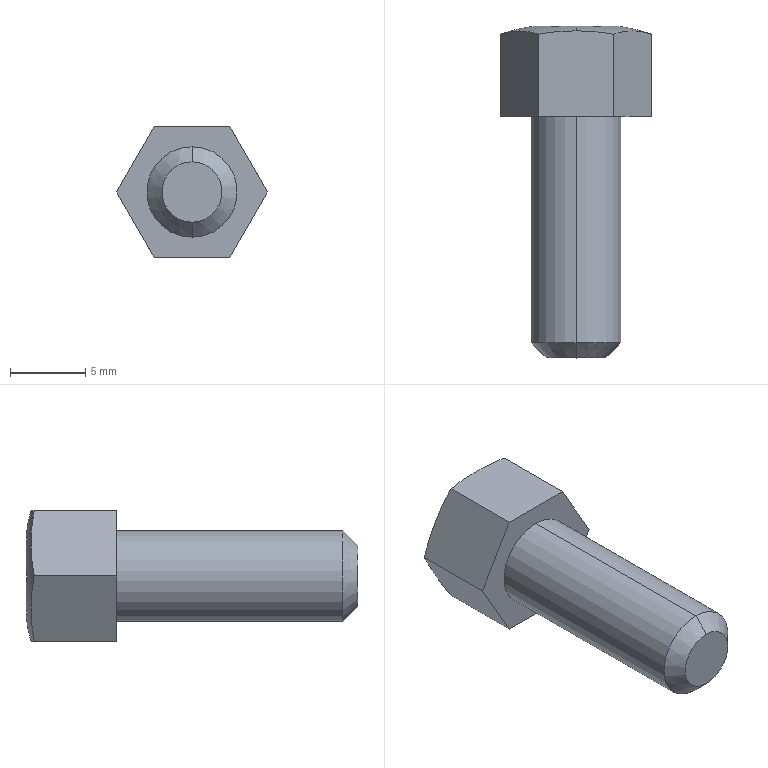Part | SolidWorks | features ICE 2, Revolution 2, BlendCut 1, Chamfer 1, Fillet 1, RevCut 1 | 1 solid | 26 faces | box 10 x 22 x 8.66 mm | volume 755.833 mm3 | plane 14 | torus 6 | cone 4 | cylinder 2 | commonest cylinder face diameters 6 x2
STEP:
#1=CARTESIAN_POINT('',(0.,19.033,-2.014));
#2=VERTEX_POINT('',#1);
#3=CARTESIAN_POINT('',(0.,19.033,2.014));
#4=VERTEX_POINT('',#3);
#5=CARTESIAN_POINT('',(0.,19.033,0.));
#6=DIRECTION('',(0.,-1.,0.));
#7=DIRECTION('',(0.,0.,1.));
#8=AXIS2_PLACEMENT_3D('',#5,#6,#7);
#9=CIRCLE('',#8,2.014);
#10=EDGE_CURVE('',#2,#4,#9,.T.);
#11=ORIENTED_EDGE('',*,*,#10,.F.);
#12=CARTESIAN_POINT('',(0.,18.76,-0.5137));
#13=VERTEX_POINT('',#12);
#14=CARTESIAN_POINT('',(0.,-0.7665,-4.841));
#15=DIRECTION('',(1.,0.,0.));
#16=DIRECTION('',(0.,0.,-1.));
#17=AXIS2_PLACEMENT_3D('',#14,#15,#16);
#18=CIRCLE('',#17,20.);
#19=EDGE_CURVE('',#2,#13,#18,.T.);
#20=ORIENTED_EDGE('',*,*,#19,.T.);
#21=CARTESIAN_POINT('',(0.,18.76,0.5137));
#22=VERTEX_POINT('',#21);
#23=CARTESIAN_POINT('',(0.,18.76,0.));
#24=DIRECTION('',(0.,1.,0.));
#25=DIRECTION('',(0.,0.,1.));
#26=AXIS2_PLACEMENT_3D('',#23,#24,#25);
#27=CIRCLE('',#26,0.5137);
#28=EDGE_CURVE('',#22,#13,#27,.T.);
#29=ORIENTED_EDGE('',*,*,#28,.F.);
#30=CARTESIAN_POINT('',(0.,-0.7665,4.841));
#31=DIRECTION('',(-1.,0.,0.));
#32=DIRECTION('',(0.,0.,1.));
#33=AXIS2_PLACEMENT_3D('',#30,#31,#32);
#34=CIRCLE('',#33,20.);
#35=EDGE_CURVE('',#4,#22,#34,.T.);
#36=ORIENTED_EDGE('',*,*,#35,.F.);
#37=EDGE_LOOP('',(#11,#20,#29,#36));
#38=FACE_OUTER_BOUND('',#37,.T.);
#39=CARTESIAN_POINT('',(0.,-0.7665,0.));
#40=DIRECTION('',(0.,1.,0.));
#41=DIRECTION('',(0.,0.,1.));
#42=AXIS2_PLACEMENT_3D('',#39,#40,#41);
#43=TOROIDAL_SURFACE('',#42,4.841,20.);
#44=ADVANCED_FACE('',(#38),#43,.T.);
#45=CARTESIAN_POINT('',(0.,18.646,0.));
#46=VERTEX_POINT('',#45);
#47=CARTESIAN_POINT('',(0.,18.646,0.));
#48=DIRECTION('',(0.,0.2164,0.9763));
#49=VECTOR('',#48,1000.);
#50=LINE('',#47,#49);
#51=EDGE_CURVE('',#46,#22,#50,.T.);
#52=ORIENTED_EDGE('',*,*,#51,.F.);
#53=CARTESIAN_POINT('',(0.,18.646,0.));
#54=DIRECTION('',(0.,0.2164,-0.9763));
#55=VECTOR('',#54,1000.);
#56=LINE('',#53,#55);
#57=EDGE_CURVE('',#46,#13,#56,.T.);
#58=ORIENTED_EDGE('',*,*,#57,.T.);
#59=CARTESIAN_POINT('',(0.,18.76,0.));
#60=DIRECTION('',(0.,1.,0.));
#61=DIRECTION('',(0.,0.,1.));
#62=AXIS2_PLACEMENT_3D('',#59,#60,#61);
#63=CIRCLE('',#62,0.5137);
#64=EDGE_CURVE('',#13,#22,#63,.T.);
#65=ORIENTED_EDGE('',*,*,#64,.T.);
#66=EDGE_LOOP('',(#52,#58,#65));
#67=FACE_OUTER_BOUND('',#66,.T.);
#68=CARTESIAN_POINT('',(0.,1018.646,0.));
#69=DIRECTION('',(0.,1.,0.));
#70=DIRECTION('',(0.,0.,1.));
#71=AXIS2_PLACEMENT_3D('',#68,#69,#70);
#72=CONICAL_SURFACE('',#71,4511.967,1.353);
#73=ADVANCED_FACE('',(#67),#72,.F.);
#74=CARTESIAN_POINT('',(0.,19.171,2.598));
#75=VERTEX_POINT('',#74);
#76=CARTESIAN_POINT('',(-1.5,19.337,2.598));
#77=VERTEX_POINT('',#76);
#78=CARTESIAN_POINT('',(0.,19.171,2.598));
#79=CARTESIAN_POINT('',(-0.2539,19.171,2.598));
#80=CARTESIAN_POINT('',(-0.5061,19.183,2.598));
#81=CARTESIAN_POINT('',(-1.006,19.236,2.598));
#82=CARTESIAN_POINT('',(-1.255,19.277,2.598));
#83=CARTESIAN_POINT('',(-1.5,19.337,2.598));
#84=B_SPLINE_CURVE_WITH_KNOTS('',3,(#78,#79,#80,#81,#82,#83),.UNSPECIFIED.,.F.,.F.,(4,2,4),(0.,0.0007542,0.001508),.UNSPECIFIED.);
#85=EDGE_CURVE('',#75,#77,#84,.T.);
#86=ORIENTED_EDGE('',*,*,#85,.F.);
#87=CARTESIAN_POINT('',(0.,22.29,1.549));
#88=DIRECTION('',(1.,0.,0.));
#89=DIRECTION('',(0.,0.,-1.));
#90=AXIS2_PLACEMENT_3D('',#87,#88,#89);
#91=CIRCLE('',#90,3.29);
#92=EDGE_CURVE('',#75,#4,#91,.T.);
#93=ORIENTED_EDGE('',*,*,#92,.T.);
#94=CARTESIAN_POINT('',(0.,19.033,0.));
#95=DIRECTION('',(0.,-1.,0.));
#96=DIRECTION('',(0.,0.,1.));
#97=AXIS2_PLACEMENT_3D('',#94,#95,#96);
#98=CIRCLE('',#97,2.014);
#99=EDGE_CURVE('',#4,#2,#98,.T.);
#100=ORIENTED_EDGE('',*,*,#99,.T.);
#101=CARTESIAN_POINT('',(0.,19.171,-2.598));
#102=VERTEX_POINT('',#101);
#103=CARTESIAN_POINT('',(0.,22.29,-1.549));
#104=DIRECTION('',(-1.,0.,0.));
#105=DIRECTION('',(0.,0.,1.));
#106=AXIS2_PLACEMENT_3D('',#103,#104,#105);
#107=CIRCLE('',#106,3.29);
#108=EDGE_CURVE('',#102,#2,#107,.T.);
#109=ORIENTED_EDGE('',*,*,#108,.F.);
#110=CARTESIAN_POINT('',(-1.5,19.337,-2.598));
#111=VERTEX_POINT('',#110);
#112=CARTESIAN_POINT('',(-1.5,19.337,-2.598));
#113=CARTESIAN_POINT('',(-1.255,19.277,-2.598));
#114=CARTESIAN_POINT('',(-1.005,19.236,-2.598));
#115=CARTESIAN_POINT('',(-0.5045,19.183,-2.598));
#116=CARTESIAN_POINT('',(-0.2517,19.171,-2.598));
#117=CARTESIAN_POINT('',(0.,19.171,-2.598));
#118=B_SPLINE_CURVE_WITH_KNOTS('',3,(#112,#113,#114,#115,#116,#117),.UNSPECIFIED.,.F.,.F.,(4,2,4),(0.02133,0.02208,0.02283),.UNSPECIFIED.);
#119=EDGE_CURVE('',#111,#102,#118,.T.);
#120=ORIENTED_EDGE('',*,*,#119,.F.);
#121=CARTESIAN_POINT('',(-3.,19.337,0.));
#122=VERTEX_POINT('',#121);
#123=CARTESIAN_POINT('',(-3.,19.337,0.));
#124=CARTESIAN_POINT('',(-2.753,19.215,-0.4282));
#125=CARTESIAN_POINT('',(-2.503,19.172,-0.8608));
#126=CARTESIAN_POINT('',(-2.001,19.171,-1.731));
#127=CARTESIAN_POINT('',(-1.746,19.216,-2.171));
#128=CARTESIAN_POINT('',(-1.5,19.337,-2.598));
#129=B_SPLINE_CURVE_WITH_KNOTS('',3,(#123,#124,#125,#126,#127,#128),.UNSPECIFIED.,.F.,.F.,(4,2,4),(0.000000234,0.001504,0.003008),.UNSPECIFIED.);
#130=EDGE_CURVE('',#122,#111,#129,.T.);
#131=ORIENTED_EDGE('',*,*,#130,.F.);
#132=CARTESIAN_POINT('',(-1.5,19.337,2.598));
#133=CARTESIAN_POINT('',(-1.747,19.215,2.17));
#134=CARTESIAN_POINT('',(-1.997,19.172,1.737));
#135=CARTESIAN_POINT('',(-2.499,19.171,0.8671));
#136=CARTESIAN_POINT('',(-2.754,19.216,0.4267));
#137=CARTESIAN_POINT('',(-3.,19.337,0.));
#138=B_SPLINE_CURVE_WITH_KNOTS('',3,(#132,#133,#134,#135,#136,#137),.UNSPECIFIED.,.F.,.F.,(4,2,4),(0.000000234,0.001504,0.003008),.UNSPECIFIED.);
#139=EDGE_CURVE('',#77,#122,#138,.T.);
#140=ORIENTED_EDGE('',*,*,#139,.F.);
#141=EDGE_LOOP('',(#86,#93,#100,#109,#120,#131,#140));
#142=FACE_OUTER_BOUND('',#141,.T.);
#143=CARTESIAN_POINT('',(0.,22.29,0.));
#144=DIRECTION('',(0.,-1.,0.));
#145=DIRECTION('',(0.,0.,-1.));
#146=AXIS2_PLACEMENT_3D('',#143,#144,#145);
#147=TOROIDAL_SURFACE('',#146,1.549,3.29);
#148=ADVANCED_FACE('',(#142),#147,.F.);
#149=CARTESIAN_POINT('',(1.5,21.953,2.598));
#150=VERTEX_POINT('',#149);
#151=CARTESIAN_POINT('',(0.,22.,2.598));
#152=VERTEX_POINT('',#151);
#153=CARTESIAN_POINT('',(1.5,21.953,2.598));
#154=CARTESIAN_POINT('',(1.251,21.97,2.598));
#155=CARTESIAN_POINT('',(1.001,21.982,2.598));
#156=CARTESIAN_POINT('',(0.5007,21.997,2.598));
#157=CARTESIAN_POINT('',(0.2509,22.,2.598));
#158=CARTESIAN_POINT('',(0.,22.,2.598));
#159=B_SPLINE_CURVE_WITH_KNOTS('',3,(#153,#154,#155,#156,#157,#158),.UNSPECIFIED.,.F.,.F.,(4,2,4),(0.06357,0.06432,0.06508),.UNSPECIFIED.);
#160=EDGE_CURVE('',#150,#152,#159,.T.);
#161=ORIENTED_EDGE('',*,*,#160,.T.);
#162=CARTESIAN_POINT('',(0.,21.671,4.33));
#163=VERTEX_POINT('',#162);
#164=CARTESIAN_POINT('',(0.,12.554,1.703));
#165=DIRECTION('',(1.,0.,0.));
#166=DIRECTION('',(0.,0.,-1.));
#167=AXIS2_PLACEMENT_3D('',#164,#165,#166);
#168=CIRCLE('',#167,9.488);
#169=EDGE_CURVE('',#152,#163,#168,.T.);
#170=ORIENTED_EDGE('',*,*,#169,.T.);
#171=CARTESIAN_POINT('',(2.5,21.451,4.33));
#172=VERTEX_POINT('',#171);
#173=CARTESIAN_POINT('',(2.5,21.451,4.33));
#174=CARTESIAN_POINT('',(2.088,21.528,4.33));
#175=CARTESIAN_POINT('',(1.673,21.582,4.33));
#176=CARTESIAN_POINT('',(0.8397,21.654,4.33));
#177=CARTESIAN_POINT('',(0.419,21.671,4.33));
#178=CARTESIAN_POINT('',(0.,21.671,4.33));
#179=B_SPLINE_CURVE_WITH_KNOTS('',3,(#173,#174,#175,#176,#177,#178),.UNSPECIFIED.,.F.,.F.,(4,2,4),(0.05844,0.05968,0.06092),.UNSPECIFIED.);
#180=EDGE_CURVE('',#172,#163,#179,.T.);
#181=ORIENTED_EDGE('',*,*,#180,.F.);
#182=CARTESIAN_POINT('',(5.,21.451,0.));
#183=VERTEX_POINT('',#182);
#184=CARTESIAN_POINT('',(5.,21.451,0.));
#185=CARTESIAN_POINT('',(4.583,21.606,0.7217));
#186=CARTESIAN_POINT('',(3.75,21.737,2.165));
#187=CARTESIAN_POINT('',(2.917,21.606,3.608));
#188=CARTESIAN_POINT('',(2.5,21.451,4.33));
#189=B_SPLINE_CURVE_WITH_KNOTS('',3,(#184,#185,#186,#187,#188),.UNSPECIFIED.,.F.,.F.,(4,1,4),(0.000000231,0.0025,0.005),.UNSPECIFIED.);
#190=EDGE_CURVE('',#183,#172,#189,.T.);
#191=ORIENTED_EDGE('',*,*,#190,.F.);
#192=CARTESIAN_POINT('',(2.5,21.451,-4.33));
#193=VERTEX_POINT('',#192);
#194=CARTESIAN_POINT('',(2.5,21.451,-4.33));
#195=CARTESIAN_POINT('',(2.917,21.606,-3.608));
#196=CARTESIAN_POINT('',(3.75,21.737,-2.165));
#197=CARTESIAN_POINT('',(4.583,21.606,-0.7217));
#198=CARTESIAN_POINT('',(5.,21.451,0.));
#199=B_SPLINE_CURVE_WITH_KNOTS('',3,(#194,#195,#196,#197,#198),.UNSPECIFIED.,.F.,.F.,(4,1,4),(0.000000231,0.0025,0.005),.UNSPECIFIED.);
#200=EDGE_CURVE('',#193,#183,#199,.T.);
#201=ORIENTED_EDGE('',*,*,#200,.F.);
#202=CARTESIAN_POINT('',(0.,21.671,-4.33));
#203=VERTEX_POINT('',#202);
#204=CARTESIAN_POINT('',(0.,21.671,-4.33));
#205=CARTESIAN_POINT('',(0.4229,21.671,-4.33));
#206=CARTESIAN_POINT('',(0.8429,21.654,-4.33));
#207=CARTESIAN_POINT('',(1.676,21.582,-4.33));
#208=CARTESIAN_POINT('',(2.09,21.527,-4.33));
#209=CARTESIAN_POINT('',(2.5,21.451,-4.33));
#210=B_SPLINE_CURVE_WITH_KNOTS('',3,(#204,#205,#206,#207,#208,#209),.UNSPECIFIED.,.F.,.F.,(4,2,4),(0.,0.001251,0.002501),.UNSPECIFIED.);
#211=EDGE_CURVE('',#203,#193,#210,.T.);
#212=ORIENTED_EDGE('',*,*,#211,.F.);
#213=CARTESIAN_POINT('',(0.,22.,-2.598));
#214=VERTEX_POINT('',#213);
#215=CARTESIAN_POINT('',(0.,12.554,-1.703));
#216=DIRECTION('',(-1.,0.,0.));
#217=DIRECTION('',(0.,0.,1.));
#218=AXIS2_PLACEMENT_3D('',#215,#216,#217);
#219=CIRCLE('',#218,9.488);
#220=EDGE_CURVE('',#214,#203,#219,.T.);
#221=ORIENTED_EDGE('',*,*,#220,.F.);
#222=CARTESIAN_POINT('',(1.5,21.953,-2.598));
#223=VERTEX_POINT('',#222);
#224=CARTESIAN_POINT('',(0.,22.,-2.598));
#225=CARTESIAN_POINT('',(0.2505,22.,-2.598));
#226=CARTESIAN_POINT('',(0.5008,21.997,-2.598));
#227=CARTESIAN_POINT('',(1.001,21.982,-2.598));
#228=CARTESIAN_POINT('',(1.251,21.97,-2.598));
#229=CARTESIAN_POINT('',(1.5,21.953,-2.598));
#230=B_SPLINE_CURVE_WITH_KNOTS('',3,(#224,#225,#226,#227,#228,#229),.UNSPECIFIED.,.F.,.F.,(4,2,4),(0.,0.00075,0.0015),.UNSPECIFIED.);
#231=EDGE_CURVE('',#214,#223,#230,.T.);
#232=ORIENTED_EDGE('',*,*,#231,.T.);
#233=CARTESIAN_POINT('',(3.,21.953,0.));
#234=VERTEX_POINT('',#233);
#235=CARTESIAN_POINT('',(1.5,21.953,-2.598));
#236=CARTESIAN_POINT('',(1.75,21.988,-2.165));
#237=CARTESIAN_POINT('',(2.25,22.012,-1.299));
#238=CARTESIAN_POINT('',(2.75,21.988,-0.433));
#239=CARTESIAN_POINT('',(3.,21.953,0.));
#240=B_SPLINE_CURVE_WITH_KNOTS('',3,(#235,#236,#237,#238,#239),.UNSPECIFIED.,.F.,.F.,(4,1,4),(0.000000231,0.0015,0.003),.UNSPECIFIED.);
#241=EDGE_CURVE('',#223,#234,#240,.T.);
#242=ORIENTED_EDGE('',*,*,#241,.T.);
#243=CARTESIAN_POINT('',(3.,21.953,0.));
#244=CARTESIAN_POINT('',(2.75,21.988,0.433));
#245=CARTESIAN_POINT('',(2.25,22.012,1.299));
#246=CARTESIAN_POINT('',(1.75,21.988,2.165));
#247=CARTESIAN_POINT('',(1.5,21.953,2.598));
#248=B_SPLINE_CURVE_WITH_KNOTS('',3,(#243,#244,#245,#246,#247),.UNSPECIFIED.,.F.,.F.,(4,1,4),(0.000000231,0.0015,0.003),.UNSPECIFIED.);
#249=EDGE_CURVE('',#234,#150,#248,.T.);
#250=ORIENTED_EDGE('',*,*,#249,.T.);
#251=EDGE_LOOP('',(#161,#170,#181,#191,#201,#212,#221,#232,#242,#250));
#252=FACE_OUTER_BOUND('',#251,.T.);
#253=CARTESIAN_POINT('',(0.,12.554,0.));
#254=DIRECTION('',(0.,-1.,0.));
#255=DIRECTION('',(0.,0.,-1.));
#256=AXIS2_PLACEMENT_3D('',#253,#254,#255);
#257=TOROIDAL_SURFACE('',#256,1.703,9.488);
#258=ADVANCED_FACE('',(#252),#257,.T.);
#259=CARTESIAN_POINT('',(0.,0.,-2.));
#260=VERTEX_POINT('',#259);
#261=CARTESIAN_POINT('',(0.,0.,2.));
#262=VERTEX_POINT('',#261);
#263=CARTESIAN_POINT('',(0.,0.,0.));
#264=DIRECTION('',(0.,-1.,0.));
#265=DIRECTION('',(0.,0.,1.));
#266=AXIS2_PLACEMENT_3D('',#263,#264,#265);
#267=CIRCLE('',#266,2.);
#268=EDGE_CURVE('',#260,#262,#267,.T.);
#269=ORIENTED_EDGE('',*,*,#268,.F.);
#270=CARTESIAN_POINT('',(0.,1.,-3.));
#271=VERTEX_POINT('',#270);
#272=CARTESIAN_POINT('',(0.,1.,-3.));
#273=DIRECTION('',(0.,0.7071,-0.7071));
#274=VECTOR('',#273,1000.);
#275=LINE('',#272,#274);
#276=EDGE_CURVE('',#260,#271,#275,.T.);
#277=ORIENTED_EDGE('',*,*,#276,.T.);
#278=CARTESIAN_POINT('',(0.,1.,3.));
#279=VERTEX_POINT('',#278);
#280=CARTESIAN_POINT('',(0.,1.,0.));
#281=DIRECTION('',(0.,1.,0.));
#282=DIRECTION('',(0.,0.,1.));
#283=AXIS2_PLACEMENT_3D('',#280,#281,#282);
#284=CIRCLE('',#283,3.);
#285=EDGE_CURVE('',#279,#271,#284,.T.);
#286=ORIENTED_EDGE('',*,*,#285,.F.);
#287=CARTESIAN_POINT('',(0.,1.,3.));
#288=DIRECTION('',(0.,0.7071,0.7071));
#289=VECTOR('',#288,1000.);
#290=LINE('',#287,#289);
#291=EDGE_CURVE('',#262,#279,#290,.T.);
#292=ORIENTED_EDGE('',*,*,#291,.F.);
#293=EDGE_LOOP('',(#269,#277,#286,#292));
#294=FACE_OUTER_BOUND('',#293,.T.);
#295=CARTESIAN_POINT('',(0.,1.,0.));
#296=DIRECTION('',(0.,1.,0.));
#297=DIRECTION('',(0.,0.,1.));
#298=AXIS2_PLACEMENT_3D('',#295,#296,#297);
#299=CONICAL_SURFACE('',#298,3.,0.7854);
#300=ADVANCED_FACE('',(#294),#299,.T.);
#301=ORIENTED_EDGE('',*,*,#285,.T.);
#302=CARTESIAN_POINT('',(0.,16.,-3.));
#303=VERTEX_POINT('',#302);
#304=CARTESIAN_POINT('',(0.,22.,-3.));
#305=DIRECTION('',(0.,1.,0.));
#306=VECTOR('',#305,1000.);
#307=LINE('',#304,#306);
#308=EDGE_CURVE('',#271,#303,#307,.T.);
#309=ORIENTED_EDGE('',*,*,#308,.T.);
#310=CARTESIAN_POINT('',(0.,16.,3.));
#311=VERTEX_POINT('',#310);
#312=CARTESIAN_POINT('',(0.,16.,0.));
#313=DIRECTION('',(0.,1.,0.));
#314=DIRECTION('',(0.,0.,1.));
#315=AXIS2_PLACEMENT_3D('',#312,#313,#314);
#316=CIRCLE('',#315,3.);
#317=EDGE_CURVE('',#311,#303,#316,.T.);
#318=ORIENTED_EDGE('',*,*,#317,.F.);
#319=CARTESIAN_POINT('',(0.,22.,3.));
#320=DIRECTION('',(0.,1.,0.));
#321=VECTOR('',#320,1000.);
#322=LINE('',#319,#321);
#323=EDGE_CURVE('',#279,#311,#322,.T.);
#324=ORIENTED_EDGE('',*,*,#323,.F.);
#325=EDGE_LOOP('',(#301,#309,#318,#324));
#326=FACE_OUTER_BOUND('',#325,.T.);
#327=CARTESIAN_POINT('',(0.,22.,0.));
#328=DIRECTION('',(0.,1.,0.));
#329=DIRECTION('',(0.,0.,1.));
#330=AXIS2_PLACEMENT_3D('',#327,#328,#329);
#331=CYLINDRICAL_SURFACE('',#330,3.);
#332=ADVANCED_FACE('',(#326),#331,.T.);
#333=CARTESIAN_POINT('',(2.5,16.,-4.33));
#334=VERTEX_POINT('',#333);
#335=CARTESIAN_POINT('',(2.5,-0.6367,-4.33));
#336=DIRECTION('',(0.,1.,0.));
#337=VECTOR('',#336,1000.);
#338=LINE('',#335,#337);
#339=EDGE_CURVE('',#334,#193,#338,.T.);
#340=ORIENTED_EDGE('',*,*,#339,.T.);
#341=ORIENTED_EDGE('',*,*,#200,.T.);
#342=CARTESIAN_POINT('',(5.,16.,0.));
#343=VERTEX_POINT('',#342);
#344=CARTESIAN_POINT('',(5.,-0.6367,0.));
#345=DIRECTION('',(0.,1.,0.));
#346=VECTOR('',#345,1000.);
#347=LINE('',#344,#346);
#348=EDGE_CURVE('',#343,#183,#347,.T.);
#349=ORIENTED_EDGE('',*,*,#348,.F.);
#350=CARTESIAN_POINT('',(5.,16.,0.));
#351=DIRECTION('',(0.5,0.,0.866));
#352=VECTOR('',#351,1000.);
#353=LINE('',#350,#352);
#354=EDGE_CURVE('',#334,#343,#353,.T.);
#355=ORIENTED_EDGE('',*,*,#354,.F.);
#356=EDGE_LOOP('',(#340,#341,#349,#355));
#357=FACE_OUTER_BOUND('',#356,.T.);
#358=CARTESIAN_POINT('',(5.,-0.6367,0.));
#359=DIRECTION('',(0.866,0.,-0.5));
#360=DIRECTION('',(-0.5,0.,-0.866));
#361=AXIS2_PLACEMENT_3D('',#358,#359,#360);
#362=PLANE('',#361);
#363=ADVANCED_FACE('',(#357),#362,.T.);
#364=CARTESIAN_POINT('',(-2.5,16.,-4.33));
#365=VERTEX_POINT('',#364);
#366=CARTESIAN_POINT('',(-2.5,21.451,-4.33));
#367=VERTEX_POINT('',#366);
#368=CARTESIAN_POINT('',(-2.5,-0.6367,-4.33));
#369=DIRECTION('',(0.,1.,0.));
#370=VECTOR('',#369,1000.);
#371=LINE('',#368,#370);
#372=EDGE_CURVE('',#365,#367,#371,.T.);
#373=ORIENTED_EDGE('',*,*,#372,.T.);
#374=CARTESIAN_POINT('',(-2.5,21.451,-4.33));
#375=CARTESIAN_POINT('',(-2.088,21.528,-4.33));
#376=CARTESIAN_POINT('',(-1.673,21.582,-4.33));
#377=CARTESIAN_POINT('',(-0.8397,21.654,-4.33));
#378=CARTESIAN_POINT('',(-0.419,21.671,-4.33));
#379=CARTESIAN_POINT('',(0.,21.671,-4.33));
#380=B_SPLINE_CURVE_WITH_KNOTS('',3,(#374,#375,#376,#377,#378,#379),.UNSPECIFIED.,.F.,.F.,(4,2,4),(0.05844,0.05968,0.06092),.UNSPECIFIED.);
#381=EDGE_CURVE('',#367,#203,#380,.T.);
#382=ORIENTED_EDGE('',*,*,#381,.T.);
#383=ORIENTED_EDGE('',*,*,#211,.T.);
#384=ORIENTED_EDGE('',*,*,#339,.F.);
#385=CARTESIAN_POINT('',(2.5,16.,-4.33));
#386=DIRECTION('',(1.,0.,0.));
#387=VECTOR('',#386,1000.);
#388=LINE('',#385,#387);
#389=EDGE_CURVE('',#365,#334,#388,.T.);
#390=ORIENTED_EDGE('',*,*,#389,.F.);
#391=EDGE_LOOP('',(#373,#382,#383,#384,#390));
#392=FACE_OUTER_BOUND('',#391,.T.);
#393=CARTESIAN_POINT('',(2.5,-0.6367,-4.33));
#394=DIRECTION('',(0.,0.,-1.));
#395=DIRECTION('',(-1.,0.,0.));
#396=AXIS2_PLACEMENT_3D('',#393,#394,#395);
#397=PLANE('',#396);
#398=ADVANCED_FACE('',(#392),#397,.T.);
#399=CARTESIAN_POINT('',(-5.,16.,0.));
#400=VERTEX_POINT('',#399);
#401=CARTESIAN_POINT('',(-5.,21.451,0.));
#402=VERTEX_POINT('',#401);
#403=CARTESIAN_POINT('',(-5.,-0.6367,0.));
#404=DIRECTION('',(0.,1.,0.));
#405=VECTOR('',#404,1000.);
#406=LINE('',#403,#405);
#407=EDGE_CURVE('',#400,#402,#406,.T.);
#408=ORIENTED_EDGE('',*,*,#407,.T.);
#409=CARTESIAN_POINT('',(-5.,21.451,0.));
#410=CARTESIAN_POINT('',(-4.583,21.606,-0.7217));
#411=CARTESIAN_POINT('',(-3.75,21.737,-2.165));
#412=CARTESIAN_POINT('',(-2.917,21.606,-3.608));
#413=CARTESIAN_POINT('',(-2.5,21.451,-4.33));
#414=B_SPLINE_CURVE_WITH_KNOTS('',3,(#409,#410,#411,#412,#413),.UNSPECIFIED.,.F.,.F.,(4,1,4),(0.000000231,0.0025,0.005),.UNSPECIFIED.);
#415=EDGE_CURVE('',#402,#367,#414,.T.);
#416=ORIENTED_EDGE('',*,*,#415,.T.);
#417=ORIENTED_EDGE('',*,*,#372,.F.);
#418=CARTESIAN_POINT('',(-2.5,16.,-4.33));
#419=DIRECTION('',(0.5,0.,-0.866));
#420=VECTOR('',#419,1000.);
#421=LINE('',#418,#420);
#422=EDGE_CURVE('',#400,#365,#421,.T.);
#423=ORIENTED_EDGE('',*,*,#422,.F.);
#424=EDGE_LOOP('',(#408,#416,#417,#423));
#425=FACE_OUTER_BOUND('',#424,.T.);
#426=CARTESIAN_POINT('',(-2.5,-0.6367,-4.33));
#427=DIRECTION('',(-0.866,0.,-0.5));
#428=DIRECTION('',(-0.5,0.,0.866));
#429=AXIS2_PLACEMENT_3D('',#426,#427,#428);
#430=PLANE('',#429);
#431=ADVANCED_FACE('',(#425),#430,.T.);
#432=CARTESIAN_POINT('',(-2.5,16.,4.33));
#433=VERTEX_POINT('',#432);
#434=CARTESIAN_POINT('',(-2.5,21.451,4.33));
#435=VERTEX_POINT('',#434);
#436=CARTESIAN_POINT('',(-2.5,-0.6367,4.33));
#437=DIRECTION('',(0.,1.,0.));
#438=VECTOR('',#437,1000.);
#439=LINE('',#436,#438);
#440=EDGE_CURVE('',#433,#435,#439,.T.);
#441=ORIENTED_EDGE('',*,*,#440,.T.);
#442=CARTESIAN_POINT('',(-2.5,21.451,4.33));
#443=CARTESIAN_POINT('',(-2.917,21.606,3.608));
#444=CARTESIAN_POINT('',(-3.75,21.737,2.165));
#445=CARTESIAN_POINT('',(-4.583,21.606,0.7217));
#446=CARTESIAN_POINT('',(-5.,21.451,0.));
#447=B_SPLINE_CURVE_WITH_KNOTS('',3,(#442,#443,#444,#445,#446),.UNSPECIFIED.,.F.,.F.,(4,1,4),(0.000000231,0.0025,0.005),.UNSPECIFIED.);
#448=EDGE_CURVE('',#435,#402,#447,.T.);
#449=ORIENTED_EDGE('',*,*,#448,.T.);
#450=ORIENTED_EDGE('',*,*,#407,.F.);
#451=CARTESIAN_POINT('',(-5.,16.,0.));
#452=DIRECTION('',(-0.5,0.,-0.866));
#453=VECTOR('',#452,1000.);
#454=LINE('',#451,#453);
#455=EDGE_CURVE('',#433,#400,#454,.T.);
#456=ORIENTED_EDGE('',*,*,#455,.F.);
#457=EDGE_LOOP('',(#441,#449,#450,#456));
#458=FACE_OUTER_BOUND('',#457,.T.);
#459=CARTESIAN_POINT('',(-5.,-0.6367,0.));
#460=DIRECTION('',(-0.866,0.,0.5));
#461=DIRECTION('',(0.5,0.,0.866));
#462=AXIS2_PLACEMENT_3D('',#459,#460,#461);
#463=PLANE('',#462);
#464=ADVANCED_FACE('',(#458),#463,.T.);
#465=CARTESIAN_POINT('',(2.5,16.,4.33));
#466=VERTEX_POINT('',#465);
#467=CARTESIAN_POINT('',(2.5,-0.6367,4.33));
#468=DIRECTION('',(0.,1.,0.));
#469=VECTOR('',#468,1000.);
#470=LINE('',#467,#469);
#471=EDGE_CURVE('',#466,#172,#470,.T.);
#472=ORIENTED_EDGE('',*,*,#471,.T.);
#473=ORIENTED_EDGE('',*,*,#180,.T.);
#474=CARTESIAN_POINT('',(0.,21.671,4.33));
#475=CARTESIAN_POINT('',(-0.4229,21.671,4.33));
#476=CARTESIAN_POINT('',(-0.8429,21.654,4.33));
#477=CARTESIAN_POINT('',(-1.676,21.582,4.33));
#478=CARTESIAN_POINT('',(-2.09,21.527,4.33));
#479=CARTESIAN_POINT('',(-2.5,21.451,4.33));
#480=B_SPLINE_CURVE_WITH_KNOTS('',3,(#474,#475,#476,#477,#478,#479),.UNSPECIFIED.,.F.,.F.,(4,2,4),(0.,0.001251,0.002501),.UNSPECIFIED.);
#481=EDGE_CURVE('',#163,#435,#480,.T.);
#482=ORIENTED_EDGE('',*,*,#481,.T.);
#483=ORIENTED_EDGE('',*,*,#440,.F.);
#484=CARTESIAN_POINT('',(-2.5,16.,4.33));
#485=DIRECTION('',(-1.,0.,0.));
#486=VECTOR('',#485,1000.);
#487=LINE('',#484,#486);
#488=EDGE_CURVE('',#466,#433,#487,.T.);
#489=ORIENTED_EDGE('',*,*,#488,.F.);
#490=EDGE_LOOP('',(#472,#473,#482,#483,#489));
#491=FACE_OUTER_BOUND('',#490,.T.);
#492=CARTESIAN_POINT('',(-2.5,-0.6367,4.33));
#493=DIRECTION('',(0.,0.,1.));
#494=DIRECTION('',(1.,0.,0.));
#495=AXIS2_PLACEMENT_3D('',#492,#493,#494);
#496=PLANE('',#495);
#497=ADVANCED_FACE('',(#491),#496,.T.);
#498=ORIENTED_EDGE('',*,*,#348,.T.);
#499=ORIENTED_EDGE('',*,*,#190,.T.);
#500=ORIENTED_EDGE('',*,*,#471,.F.);
#501=CARTESIAN_POINT('',(2.5,16.,4.33));
#502=DIRECTION('',(-0.5,0.,0.866));
#503=VECTOR('',#502,1000.);
#504=LINE('',#501,#503);
#505=EDGE_CURVE('',#343,#466,#504,.T.);
#506=ORIENTED_EDGE('',*,*,#505,.F.);
#507=EDGE_LOOP('',(#498,#499,#500,#506));
#508=FACE_OUTER_BOUND('',#507,.T.);
#509=CARTESIAN_POINT('',(2.5,-0.6367,4.33));
#510=DIRECTION('',(0.866,0.,0.5));
#511=DIRECTION('',(0.5,0.,-0.866));
#512=AXIS2_PLACEMENT_3D('',#509,#510,#511);
#513=PLANE('',#512);
#514=ADVANCED_FACE('',(#508),#513,.T.);
#515=ORIENTED_EDGE('',*,*,#317,.T.);
#516=CARTESIAN_POINT('',(0.,16.,0.));
#517=DIRECTION('',(0.,1.,0.));
#518=DIRECTION('',(0.,0.,1.));
#519=AXIS2_PLACEMENT_3D('',#516,#517,#518);
#520=CIRCLE('',#519,3.);
#521=EDGE_CURVE('',#303,#311,#520,.T.);
#522=ORIENTED_EDGE('',*,*,#521,.T.);
#523=EDGE_LOOP('',(#515,#522));
#524=FACE_BOUND('',#523,.T.);
#525=ORIENTED_EDGE('',*,*,#354,.T.);
#526=ORIENTED_EDGE('',*,*,#505,.T.);
#527=ORIENTED_EDGE('',*,*,#488,.T.);
#528=ORIENTED_EDGE('',*,*,#455,.T.);
#529=ORIENTED_EDGE('',*,*,#422,.T.);
#530=ORIENTED_EDGE('',*,*,#389,.T.);
#531=EDGE_LOOP('',(#525,#526,#527,#528,#529,#530));
#532=FACE_OUTER_BOUND('',#531,.T.);
#533=CARTESIAN_POINT('',(3.,16.,0.));
#534=DIRECTION('',(0.,1.,0.));
#535=DIRECTION('',(0.,0.,1.));
#536=AXIS2_PLACEMENT_3D('',#533,#534,#535);
#537=PLANE('',#536);
#538=ADVANCED_FACE('',(#524,#532),#537,.F.);
#539=CARTESIAN_POINT('',(0.,0.,0.));
#540=DIRECTION('',(0.,-1.,0.));
#541=DIRECTION('',(0.,0.,1.));
#542=AXIS2_PLACEMENT_3D('',#539,#540,#541);
#543=CIRCLE('',#542,2.);
#544=EDGE_CURVE('',#262,#260,#543,.T.);
#545=ORIENTED_EDGE('',*,*,#544,.T.);
#546=ORIENTED_EDGE('',*,*,#268,.T.);
#547=EDGE_LOOP('',(#545,#546));
#548=FACE_OUTER_BOUND('',#547,.T.);
#549=CARTESIAN_POINT('',(0.,0.,0.));
#550=DIRECTION('',(0.,1.,0.));
#551=DIRECTION('',(0.,0.,1.));
#552=AXIS2_PLACEMENT_3D('',#549,#550,#551);
#553=PLANE('',#552);
#554=ADVANCED_FACE('',(#548),#553,.F.);
#555=ORIENTED_EDGE('',*,*,#308,.F.);
#556=CARTESIAN_POINT('',(0.,1.,0.));
#557=DIRECTION('',(0.,1.,0.));
#558=DIRECTION('',(0.,0.,1.));
#559=AXIS2_PLACEMENT_3D('',#556,#557,#558);
#560=CIRCLE('',#559,3.);
#561=EDGE_CURVE('',#271,#279,#560,.T.);
#562=ORIENTED_EDGE('',*,*,#561,.T.);
#563=ORIENTED_EDGE('',*,*,#323,.T.);
#564=ORIENTED_EDGE('',*,*,#521,.F.);
#565=EDGE_LOOP('',(#555,#562,#563,#564));
#566=FACE_OUTER_BOUND('',#565,.T.);
#567=CARTESIAN_POINT('',(0.,22.,0.));
#568=DIRECTION('',(0.,1.,0.));
#569=DIRECTION('',(0.,0.,1.));
#570=AXIS2_PLACEMENT_3D('',#567,#568,#569);
#571=CYLINDRICAL_SURFACE('',#570,3.);
#572=ADVANCED_FACE('',(#566),#571,.T.);
#573=ORIENTED_EDGE('',*,*,#276,.F.);
#574=ORIENTED_EDGE('',*,*,#544,.F.);
#575=ORIENTED_EDGE('',*,*,#291,.T.);
#576=ORIENTED_EDGE('',*,*,#561,.F.);
#577=EDGE_LOOP('',(#573,#574,#575,#576));
#578=FACE_OUTER_BOUND('',#577,.T.);
#579=CARTESIAN_POINT('',(0.,1.,0.));
#580=DIRECTION('',(0.,1.,0.));
#581=DIRECTION('',(0.,0.,1.));
#582=AXIS2_PLACEMENT_3D('',#579,#580,#581);
#583=CONICAL_SURFACE('',#582,3.,0.7854);
#584=ADVANCED_FACE('',(#578),#583,.T.);
#585=ORIENTED_EDGE('',*,*,#169,.F.);
#586=CARTESIAN_POINT('',(-1.5,21.953,2.598));
#587=VERTEX_POINT('',#586);
#588=CARTESIAN_POINT('',(0.,22.,2.598));
#589=CARTESIAN_POINT('',(-0.2505,22.,2.598));
#590=CARTESIAN_POINT('',(-0.5008,21.997,2.598));
#591=CARTESIAN_POINT('',(-1.001,21.982,2.598));
#592=CARTESIAN_POINT('',(-1.251,21.97,2.598));
#593=CARTESIAN_POINT('',(-1.5,21.953,2.598));
#594=B_SPLINE_CURVE_WITH_KNOTS('',3,(#588,#589,#590,#591,#592,#593),.UNSPECIFIED.,.F.,.F.,(4,2,4),(0.,0.00075,0.0015),.UNSPECIFIED.);
#595=EDGE_CURVE('',#152,#587,#594,.T.);
#596=ORIENTED_EDGE('',*,*,#595,.T.);
#597=CARTESIAN_POINT('',(-3.,21.953,0.));
#598=VERTEX_POINT('',#597);
#599=CARTESIAN_POINT('',(-1.5,21.953,2.598));
#600=CARTESIAN_POINT('',(-1.75,21.988,2.165));
#601=CARTESIAN_POINT('',(-2.25,22.012,1.299));
#602=CARTESIAN_POINT('',(-2.75,21.988,0.433));
#603=CARTESIAN_POINT('',(-3.,21.953,0.));
#604=B_SPLINE_CURVE_WITH_KNOTS('',3,(#599,#600,#601,#602,#603),.UNSPECIFIED.,.F.,.F.,(4,1,4),(0.000000231,0.0015,0.003),.UNSPECIFIED.);
#605=EDGE_CURVE('',#587,#598,#604,.T.);
#606=ORIENTED_EDGE('',*,*,#605,.T.);
#607=CARTESIAN_POINT('',(-1.5,21.953,-2.598));
#608=VERTEX_POINT('',#607);
#609=CARTESIAN_POINT('',(-3.,21.953,0.));
#610=CARTESIAN_POINT('',(-2.75,21.988,-0.433));
#611=CARTESIAN_POINT('',(-2.25,22.012,-1.299));
#612=CARTESIAN_POINT('',(-1.75,21.988,-2.165));
#613=CARTESIAN_POINT('',(-1.5,21.953,-2.598));
#614=B_SPLINE_CURVE_WITH_KNOTS('',3,(#609,#610,#611,#612,#613),.UNSPECIFIED.,.F.,.F.,(4,1,4),(0.000000231,0.0015,0.003),.UNSPECIFIED.);
#615=EDGE_CURVE('',#598,#608,#614,.T.);
#616=ORIENTED_EDGE('',*,*,#615,.T.);
#617=CARTESIAN_POINT('',(-1.5,21.953,-2.598));
#618=CARTESIAN_POINT('',(-1.251,21.97,-2.598));
#619=CARTESIAN_POINT('',(-1.001,21.982,-2.598));
#620=CARTESIAN_POINT('',(-0.5007,21.997,-2.598));
#621=CARTESIAN_POINT('',(-0.2509,22.,-2.598));
#622=CARTESIAN_POINT('',(0.,22.,-2.598));
#623=B_SPLINE_CURVE_WITH_KNOTS('',3,(#617,#618,#619,#620,#621,#622),.UNSPECIFIED.,.F.,.F.,(4,2,4),(0.06357,0.06432,0.06508),.UNSPECIFIED.);
#624=EDGE_CURVE('',#608,#214,#623,.T.);
#625=ORIENTED_EDGE('',*,*,#624,.T.);
#626=ORIENTED_EDGE('',*,*,#220,.T.);
#627=ORIENTED_EDGE('',*,*,#381,.F.);
#628=ORIENTED_EDGE('',*,*,#415,.F.);
#629=ORIENTED_EDGE('',*,*,#448,.F.);
#630=ORIENTED_EDGE('',*,*,#481,.F.);
#631=EDGE_LOOP('',(#585,#596,#606,#616,#625,#626,#627,#628,#629,#630));
#632=FACE_OUTER_BOUND('',#631,.T.);
#633=CARTESIAN_POINT('',(0.,12.554,0.));
#634=DIRECTION('',(0.,-1.,0.));
#635=DIRECTION('',(0.,0.,-1.));
#636=AXIS2_PLACEMENT_3D('',#633,#634,#635);
#637=TOROIDAL_SURFACE('',#636,1.703,9.488);
#638=ADVANCED_FACE('',(#632),#637,.T.);
#639=CARTESIAN_POINT('',(1.5,19.337,-2.598));
#640=VERTEX_POINT('',#639);
#641=CARTESIAN_POINT('',(1.5,19.,-2.598));
#642=DIRECTION('',(0.,1.,0.));
#643=VECTOR('',#642,1000.);
#644=LINE('',#641,#643);
#645=EDGE_CURVE('',#640,#223,#644,.T.);
#646=ORIENTED_EDGE('',*,*,#645,.F.);
#647=CARTESIAN_POINT('',(3.,19.337,0.));
#648=VERTEX_POINT('',#647);
#649=CARTESIAN_POINT('',(1.5,19.337,-2.598));
#650=CARTESIAN_POINT('',(1.747,19.215,-2.17));
#651=CARTESIAN_POINT('',(1.997,19.172,-1.737));
#652=CARTESIAN_POINT('',(2.499,19.171,-0.8671));
#653=CARTESIAN_POINT('',(2.754,19.216,-0.4267));
#654=CARTESIAN_POINT('',(3.,19.337,0.));
#655=B_SPLINE_CURVE_WITH_KNOTS('',3,(#649,#650,#651,#652,#653,#654),.UNSPECIFIED.,.F.,.F.,(4,2,4),(0.000000234,0.001504,0.003008),.UNSPECIFIED.);
#656=EDGE_CURVE('',#640,#648,#655,.T.);
#657=ORIENTED_EDGE('',*,*,#656,.T.);
#658=CARTESIAN_POINT('',(3.,19.,0.));
#659=DIRECTION('',(0.,1.,0.));
#660=VECTOR('',#659,1000.);
#661=LINE('',#658,#660);
#662=EDGE_CURVE('',#648,#234,#661,.T.);
#663=ORIENTED_EDGE('',*,*,#662,.T.);
#664=ORIENTED_EDGE('',*,*,#241,.F.);
#665=EDGE_LOOP('',(#646,#657,#663,#664));
#666=FACE_OUTER_BOUND('',#665,.T.);
#667=CARTESIAN_POINT('',(3.,19.,0.));
#668=DIRECTION('',(0.866,0.,-0.5));
#669=DIRECTION('',(-0.5,0.,-0.866));
#670=AXIS2_PLACEMENT_3D('',#667,#668,#669);
#671=PLANE('',#670);
#672=ADVANCED_FACE('',(#666),#671,.F.);
#673=CARTESIAN_POINT('',(-1.5,19.,-2.598));
#674=DIRECTION('',(0.,1.,0.));
#675=VECTOR('',#674,1000.);
#676=LINE('',#673,#675);
#677=EDGE_CURVE('',#111,#608,#676,.T.);
#678=ORIENTED_EDGE('',*,*,#677,.F.);
#679=ORIENTED_EDGE('',*,*,#119,.T.);
#680=CARTESIAN_POINT('',(0.,19.171,-2.598));
#681=CARTESIAN_POINT('',(0.2539,19.171,-2.598));
#682=CARTESIAN_POINT('',(0.5061,19.183,-2.598));
#683=CARTESIAN_POINT('',(1.006,19.236,-2.598));
#684=CARTESIAN_POINT('',(1.255,19.277,-2.598));
#685=CARTESIAN_POINT('',(1.5,19.337,-2.598));
#686=B_SPLINE_CURVE_WITH_KNOTS('',3,(#680,#681,#682,#683,#684,#685),.UNSPECIFIED.,.F.,.F.,(4,2,4),(0.,0.0007542,0.001508),.UNSPECIFIED.);
#687=EDGE_CURVE('',#102,#640,#686,.T.);
#688=ORIENTED_EDGE('',*,*,#687,.T.);
#689=ORIENTED_EDGE('',*,*,#645,.T.);
#690=ORIENTED_EDGE('',*,*,#231,.F.);
#691=ORIENTED_EDGE('',*,*,#624,.F.);
#692=EDGE_LOOP('',(#678,#679,#688,#689,#690,#691));
#693=FACE_OUTER_BOUND('',#692,.T.);
#694=CARTESIAN_POINT('',(1.5,19.,-2.598));
#695=DIRECTION('',(0.,0.,-1.));
#696=DIRECTION('',(-1.,0.,0.));
#697=AXIS2_PLACEMENT_3D('',#694,#695,#696);
#698=PLANE('',#697);
#699=ADVANCED_FACE('',(#693),#698,.F.);
#700=CARTESIAN_POINT('',(-3.,19.,0.));
#701=DIRECTION('',(0.,1.,0.));
#702=VECTOR('',#701,1000.);
#703=LINE('',#700,#702);
#704=EDGE_CURVE('',#122,#598,#703,.T.);
#705=ORIENTED_EDGE('',*,*,#704,.F.);
#706=ORIENTED_EDGE('',*,*,#130,.T.);
#707=ORIENTED_EDGE('',*,*,#677,.T.);
#708=ORIENTED_EDGE('',*,*,#615,.F.);
#709=EDGE_LOOP('',(#705,#706,#707,#708));
#710=FACE_OUTER_BOUND('',#709,.T.);
#711=CARTESIAN_POINT('',(-1.5,19.,-2.598));
#712=DIRECTION('',(-0.866,0.,-0.5));
#713=DIRECTION('',(-0.5,0.,0.866));
#714=AXIS2_PLACEMENT_3D('',#711,#712,#713);
#715=PLANE('',#714);
#716=ADVANCED_FACE('',(#710),#715,.F.);
#717=CARTESIAN_POINT('',(-1.5,19.,2.598));
#718=DIRECTION('',(0.,1.,0.));
#719=VECTOR('',#718,1000.);
#720=LINE('',#717,#719);
#721=EDGE_CURVE('',#77,#587,#720,.T.);
#722=ORIENTED_EDGE('',*,*,#721,.F.);
#723=ORIENTED_EDGE('',*,*,#139,.T.);
#724=ORIENTED_EDGE('',*,*,#704,.T.);
#725=ORIENTED_EDGE('',*,*,#605,.F.);
#726=EDGE_LOOP('',(#722,#723,#724,#725));
#727=FACE_OUTER_BOUND('',#726,.T.);
#728=CARTESIAN_POINT('',(-3.,19.,0.));
#729=DIRECTION('',(-0.866,0.,0.5));
#730=DIRECTION('',(0.5,0.,0.866));
#731=AXIS2_PLACEMENT_3D('',#728,#729,#730);
#732=PLANE('',#731);
#733=ADVANCED_FACE('',(#727),#732,.F.);
#734=CARTESIAN_POINT('',(1.5,19.337,2.598));
#735=VERTEX_POINT('',#734);
#736=CARTESIAN_POINT('',(1.5,19.,2.598));
#737=DIRECTION('',(0.,1.,0.));
#738=VECTOR('',#737,1000.);
#739=LINE('',#736,#738);
#740=EDGE_CURVE('',#735,#150,#739,.T.);
#741=ORIENTED_EDGE('',*,*,#740,.F.);
#742=CARTESIAN_POINT('',(1.5,19.337,2.598));
#743=CARTESIAN_POINT('',(1.255,19.277,2.598));
#744=CARTESIAN_POINT('',(1.005,19.236,2.598));
#745=CARTESIAN_POINT('',(0.5045,19.183,2.598));
#746=CARTESIAN_POINT('',(0.2517,19.171,2.598));
#747=CARTESIAN_POINT('',(0.,19.171,2.598));
#748=B_SPLINE_CURVE_WITH_KNOTS('',3,(#742,#743,#744,#745,#746,#747),.UNSPECIFIED.,.F.,.F.,(4,2,4),(0.02133,0.02208,0.02283),.UNSPECIFIED.);
#749=EDGE_CURVE('',#735,#75,#748,.T.);
#750=ORIENTED_EDGE('',*,*,#749,.T.);
#751=ORIENTED_EDGE('',*,*,#85,.T.);
#752=ORIENTED_EDGE('',*,*,#721,.T.);
#753=ORIENTED_EDGE('',*,*,#595,.F.);
#754=ORIENTED_EDGE('',*,*,#160,.F.);
#755=EDGE_LOOP('',(#741,#750,#751,#752,#753,#754));
#756=FACE_OUTER_BOUND('',#755,.T.);
#757=CARTESIAN_POINT('',(-1.5,19.,2.598));
#758=DIRECTION('',(0.,0.,1.));
#759=DIRECTION('',(1.,0.,0.));
#760=AXIS2_PLACEMENT_3D('',#757,#758,#759);
#761=PLANE('',#760);
#762=ADVANCED_FACE('',(#756),#761,.F.);
#763=ORIENTED_EDGE('',*,*,#662,.F.);
#764=CARTESIAN_POINT('',(3.,19.337,0.));
#765=CARTESIAN_POINT('',(2.753,19.215,0.4282));
#766=CARTESIAN_POINT('',(2.503,19.172,0.8608));
#767=CARTESIAN_POINT('',(2.001,19.171,1.731));
#768=CARTESIAN_POINT('',(1.746,19.216,2.171));
#769=CARTESIAN_POINT('',(1.5,19.337,2.598));
#770=B_SPLINE_CURVE_WITH_KNOTS('',3,(#764,#765,#766,#767,#768,#769),.UNSPECIFIED.,.F.,.F.,(4,2,4),(0.000000234,0.001504,0.003008),.UNSPECIFIED.);
#771=EDGE_CURVE('',#648,#735,#770,.T.);
#772=ORIENTED_EDGE('',*,*,#771,.T.);
#773=ORIENTED_EDGE('',*,*,#740,.T.);
#774=ORIENTED_EDGE('',*,*,#249,.F.);
#775=EDGE_LOOP('',(#763,#772,#773,#774));
#776=FACE_OUTER_BOUND('',#775,.T.);
#777=CARTESIAN_POINT('',(1.5,19.,2.598));
#778=DIRECTION('',(0.866,0.,0.5));
#779=DIRECTION('',(0.5,0.,-0.866));
#780=AXIS2_PLACEMENT_3D('',#777,#778,#779);
#781=PLANE('',#780);
#782=ADVANCED_FACE('',(#776),#781,.F.);
#783=ORIENTED_EDGE('',*,*,#92,.F.);
#784=ORIENTED_EDGE('',*,*,#749,.F.);
#785=ORIENTED_EDGE('',*,*,#771,.F.);
#786=ORIENTED_EDGE('',*,*,#656,.F.);
#787=ORIENTED_EDGE('',*,*,#687,.F.);
#788=ORIENTED_EDGE('',*,*,#108,.T.);
#789=ORIENTED_EDGE('',*,*,#10,.T.);
#790=EDGE_LOOP('',(#783,#784,#785,#786,#787,#788,#789));
#791=FACE_OUTER_BOUND('',#790,.T.);
#792=CARTESIAN_POINT('',(0.,22.29,0.));
#793=DIRECTION('',(0.,-1.,0.));
#794=DIRECTION('',(0.,0.,-1.));
#795=AXIS2_PLACEMENT_3D('',#792,#793,#794);
#796=TOROIDAL_SURFACE('',#795,1.549,3.29);
#797=ADVANCED_FACE('',(#791),#796,.F.);
#798=ORIENTED_EDGE('',*,*,#57,.F.);
#799=ORIENTED_EDGE('',*,*,#51,.T.);
#800=ORIENTED_EDGE('',*,*,#28,.T.);
#801=EDGE_LOOP('',(#798,#799,#800));
#802=FACE_OUTER_BOUND('',#801,.T.);
#803=CARTESIAN_POINT('',(0.,1018.646,0.));
#804=DIRECTION('',(0.,1.,0.));
#805=DIRECTION('',(0.,0.,1.));
#806=AXIS2_PLACEMENT_3D('',#803,#804,#805);
#807=CONICAL_SURFACE('',#806,4511.967,1.353);
#808=ADVANCED_FACE('',(#802),#807,.F.);
#809=ORIENTED_EDGE('',*,*,#19,.F.);
#810=ORIENTED_EDGE('',*,*,#99,.F.);
#811=ORIENTED_EDGE('',*,*,#35,.T.);
#812=ORIENTED_EDGE('',*,*,#64,.F.);
#813=EDGE_LOOP('',(#809,#810,#811,#812));
#814=FACE_OUTER_BOUND('',#813,.T.);
#815=CARTESIAN_POINT('',(0.,-0.7665,0.));
#816=DIRECTION('',(0.,1.,0.));
#817=DIRECTION('',(0.,0.,1.));
#818=AXIS2_PLACEMENT_3D('',#815,#816,#817);
#819=TOROIDAL_SURFACE('',#818,4.841,20.);
#820=ADVANCED_FACE('',(#814),#819,.T.);
#821=CLOSED_SHELL('',(#44,#73,#148,#258,#300,#332,#363,#398,#431,#464,#497,#514,#538,#554,#572,#584,#638,#672,#699,#716,#733,#762,#782,#797,#808,#820));
#822=MANIFOLD_SOLID_BREP('',#821);
#823=CARTESIAN_POINT('',(0.,0.,0.));
#824=DIRECTION('',(0.,0.,1.));
#825=DIRECTION('',(1.,0.,0.));
#826=AXIS2_PLACEMENT_3D('',#823,#824,#825);
#827=(LENGTH_UNIT()NAMED_UNIT(*)SI_UNIT(.MILLI.,.METRE.));
#828=UNCERTAINTY_MEASURE_WITH_UNIT(LENGTH_MEASURE(0.00001),#827,'','');
#829=(NAMED_UNIT(*)PLANE_ANGLE_UNIT()SI_UNIT($,.RADIAN.));
#830=(NAMED_UNIT(*)SI_UNIT($,.STERADIAN.)SOLID_ANGLE_UNIT());
#831=(GEOMETRIC_REPRESENTATION_CONTEXT(3)GLOBAL_UNCERTAINTY_ASSIGNED_CONTEXT((#828))GLOBAL_UNIT_ASSIGNED_CONTEXT((#827,#829,#830))REPRESENTATION_CONTEXT('',''));
#832=ADVANCED_BREP_SHAPE_REPRESENTATION('',(#822,#826),#831);